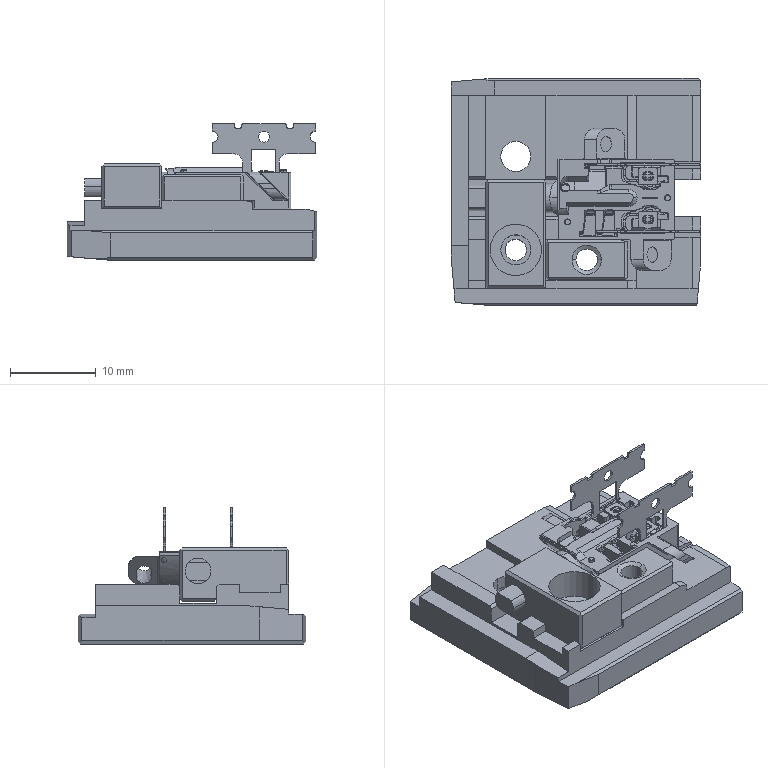Part | NX | 7 solids | 1083 faces | box 29 x 26.5 x 15.878 mm | volume 4428 mm3 | plane 596 | cylinder 327 | torus 62 | sphere 48 | cone 28 | spline 22 | commonest cylinder face diameters 0.2 x110 0.3 x32 0.4 x20 0.7 x18 1 x16 1.3 x12